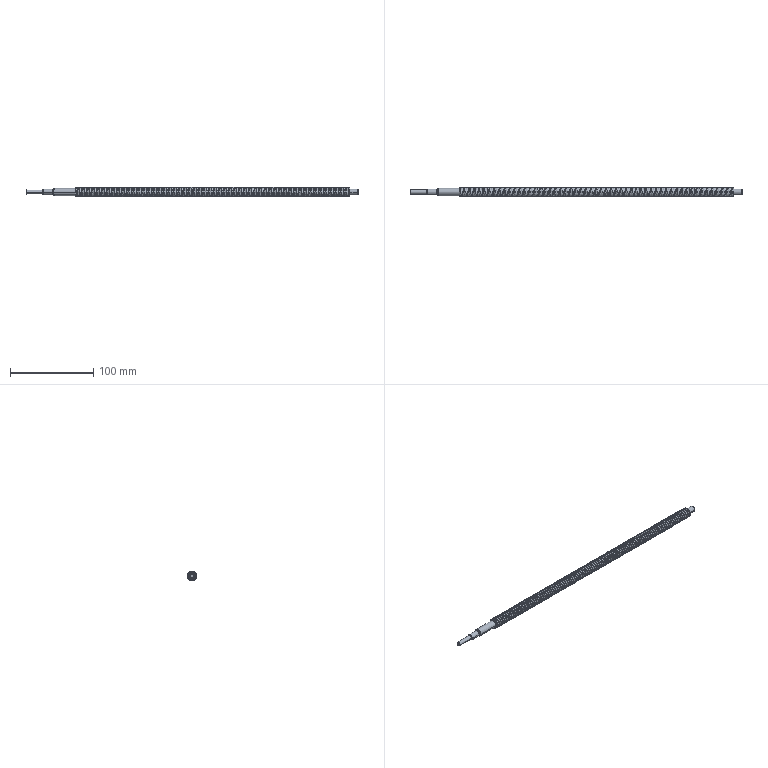Part | Creo | features DATUM PLANE 3, COORDINATE SYSTEM 1, CURVE 1, CUT 1, PROTRUSION 1 | 1 solid | 275 faces | box 399.5 x 12 x 12.003 mm | volume 34208 mm3 | cylinder 230 | spline 28 | cone 10 | plane 7 | commonest cylinder face diameters 12 x220 7 x4 5 x2 6 x2 9 x2